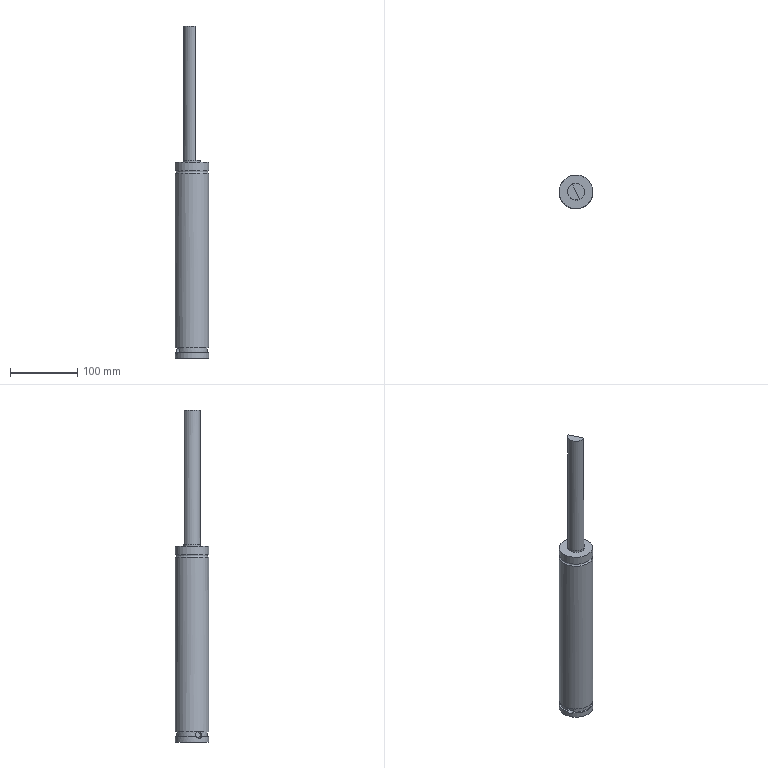Part | NX | features MAIN_BODY 2 | 1 solid | 16 faces | box 50.2 x 50.2 x 495 mm | volume 624869 mm3 | plane 8 | cylinder 7 | torus 1 | commonest cylinder face diameters 50.2 x3 9.72 x1 24.98 x1 25 x1 46.2 x1
STEP:
#1=CARTESIAN_POINT('',(178.732,295.899,-605.));
#2=VERTEX_POINT('',#1);
#3=CARTESIAN_POINT('',(177.181,299.227,-605.));
#4=VERTEX_POINT('',#3);
#5=CARTESIAN_POINT('',(200.644,308.142,-605.));
#6=DIRECTION('',(0.,0.,-1.));
#7=DIRECTION('',(0.9063,0.4226,0.));
#8=AXIS2_PLACEMENT_3D('',#5,#6,#7);
#9=CIRCLE('',#8,25.1);
#10=EDGE_CURVE('',#2,#4,#9,.F.);
#11=ORIENTED_EDGE('',*,*,#10,.T.);
#12=CARTESIAN_POINT('',(177.181,299.227,-605.));
#13=CARTESIAN_POINT('',(177.597,298.13,-604.523));
#14=CARTESIAN_POINT('',(178.16,296.923,-604.523));
#15=CARTESIAN_POINT('',(178.732,295.899,-605.));
#16=B_SPLINE_CURVE_WITH_KNOTS('',3,(#12,#13,#14,#15),.UNSPECIFIED.,.F.,.F.,(4,4),(0.,0.003746),.UNSPECIFIED.);
#17=EDGE_CURVE('',#4,#2,#16,.T.);
#18=ORIENTED_EDGE('',*,*,#17,.T.);
#19=EDGE_LOOP('',(#11,#18));
#20=FACE_BOUND('',#19,.T.);
#21=CARTESIAN_POINT('',(223.392,318.75,-344.5));
#22=VERTEX_POINT('',#21);
#23=CARTESIAN_POINT('',(200.644,308.142,-344.5));
#24=DIRECTION('',(0.,0.,-1.));
#25=DIRECTION('',(0.9063,0.4226,0.));
#26=AXIS2_PLACEMENT_3D('',#23,#24,#25);
#27=CIRCLE('',#26,25.1);
#28=EDGE_CURVE('',#22,#22,#27,.T.);
#29=ORIENTED_EDGE('',*,*,#28,.T.);
#30=EDGE_LOOP('',(#29));
#31=FACE_BOUND('',#30,.T.);
#32=CARTESIAN_POINT('',(200.644,308.142,-328.));
#33=DIRECTION('',(0.,0.,-1.));
#34=DIRECTION('',(0.9063,0.4226,0.));
#35=AXIS2_PLACEMENT_3D('',#32,#33,#34);
#36=CYLINDRICAL_SURFACE('',#35,25.1);
#37=ADVANCED_FACE('',(#20,#31),#36,.T.);
#38=CARTESIAN_POINT('',(177.896,297.535,-328.));
#39=VERTEX_POINT('',#38);
#40=CARTESIAN_POINT('',(200.644,308.142,-328.));
#41=DIRECTION('',(0.,0.,1.));
#42=DIRECTION('',(-0.9063,-0.4226,0.));
#43=AXIS2_PLACEMENT_3D('',#40,#41,#42);
#44=CIRCLE('',#43,25.1);
#45=EDGE_CURVE('',#39,#39,#44,.T.);
#46=ORIENTED_EDGE('',*,*,#45,.T.);
#47=EDGE_LOOP('',(#46));
#48=FACE_BOUND('',#47,.T.);
#49=CARTESIAN_POINT('',(189.315,302.86,-328.));
#50=VERTEX_POINT('',#49);
#51=CARTESIAN_POINT('',(200.644,308.142,-328.));
#52=DIRECTION('',(0.,0.,1.));
#53=DIRECTION('',(-0.9063,-0.4226,0.));
#54=AXIS2_PLACEMENT_3D('',#51,#52,#53);
#55=CIRCLE('',#54,12.5);
#56=EDGE_CURVE('',#50,#50,#55,.T.);
#57=ORIENTED_EDGE('',*,*,#56,.F.);
#58=EDGE_LOOP('',(#57));
#59=FACE_BOUND('',#58,.T.);
#60=CARTESIAN_POINT('',(200.644,308.142,-328.));
#61=DIRECTION('',(0.,0.,1.));
#62=DIRECTION('',(-0.9063,-0.4226,0.));
#63=AXIS2_PLACEMENT_3D('',#60,#61,#62);
#64=PLANE('',#63);
#65=ADVANCED_FACE('',(#48,#59),#64,.T.);
#66=CARTESIAN_POINT('',(223.392,318.75,-340.5));
#67=VERTEX_POINT('',#66);
#68=CARTESIAN_POINT('',(200.644,308.142,-340.5));
#69=DIRECTION('',(0.,0.,-1.));
#70=DIRECTION('',(0.9063,0.4226,0.));
#71=AXIS2_PLACEMENT_3D('',#68,#69,#70);
#72=CIRCLE('',#71,25.1);
#73=EDGE_CURVE('',#67,#67,#72,.F.);
#74=ORIENTED_EDGE('',*,*,#73,.T.);
#75=EDGE_LOOP('',(#74));
#76=FACE_BOUND('',#75,.T.);
#77=ORIENTED_EDGE('',*,*,#45,.F.);
#78=EDGE_LOOP('',(#77));
#79=FACE_BOUND('',#78,.T.);
#80=CARTESIAN_POINT('',(200.644,308.142,-328.));
#81=DIRECTION('',(0.,0.,-1.));
#82=DIRECTION('',(0.9063,0.4226,0.));
#83=AXIS2_PLACEMENT_3D('',#80,#81,#82);
#84=CYLINDRICAL_SURFACE('',#83,25.1);
#85=ADVANCED_FACE('',(#76,#79),#84,.T.);
#86=CARTESIAN_POINT('',(195.363,319.467,-325.));
#87=VERTEX_POINT('',#86);
#88=CARTESIAN_POINT('',(205.925,296.818,-325.));
#89=VERTEX_POINT('',#88);
#90=CARTESIAN_POINT('',(205.927,296.813,-325.));
#91=CARTESIAN_POINT('',(202.961,295.43,-325.));
#92=CARTESIAN_POINT('',(195.91,295.127,-325.));
#93=CARTESIAN_POINT('',(188.088,302.287,-325.));
#94=CARTESIAN_POINT('',(187.63,312.882,-325.));
#95=CARTESIAN_POINT('',(192.395,318.088,-325.));
#96=CARTESIAN_POINT('',(195.361,319.471,-325.));
#97=B_SPLINE_CURVE_WITH_KNOTS('',3,(#90,#91,#92,#93,#94,#95,#96),.UNSPECIFIED.,.F.,.F.,(4,1,1,1,4),(0.75,0.875,1.,1.125,1.25),.UNSPECIFIED.);
#98=EDGE_CURVE('',#87,#89,#97,.F.);
#99=ORIENTED_EDGE('',*,*,#98,.F.);
#100=CARTESIAN_POINT('',(195.365,319.462,-325.));
#101=CARTESIAN_POINT('',(196.867,320.162,-325.));
#102=CARTESIAN_POINT('',(200.075,320.939,-325.));
#103=CARTESIAN_POINT('',(206.686,319.944,-325.));
#104=CARTESIAN_POINT('',(213.188,313.992,-325.));
#105=CARTESIAN_POINT('',(213.569,305.185,-325.));
#106=CARTESIAN_POINT('',(210.081,299.481,-325.));
#107=CARTESIAN_POINT('',(207.424,297.523,-325.));
#108=CARTESIAN_POINT('',(205.922,296.822,-325.));
#109=B_SPLINE_CURVE_WITH_KNOTS('',3,(#100,#101,#102,#103,#104,#105,#106,#107,#108),.UNSPECIFIED.,.F.,.F.,(4,1,1,1,1,1,4),(0.,0.125,0.25,0.5,0.75,0.875,1.),.UNSPECIFIED.);
#110=EDGE_CURVE('',#87,#89,#109,.T.);
#111=ORIENTED_EDGE('',*,*,#110,.T.);
#112=EDGE_LOOP('',(#99,#111));
#113=FACE_BOUND('',#112,.T.);
#114=ORIENTED_EDGE('',*,*,#56,.T.);
#115=EDGE_LOOP('',(#114));
#116=FACE_BOUND('',#115,.T.);
#117=CARTESIAN_POINT('',(200.644,308.142,-325.));
#118=DIRECTION('',(0.,0.,-1.));
#119=DIRECTION('',(0.9063,0.4226,0.));
#120=AXIS2_PLACEMENT_3D('',#117,#118,#119);
#121=CYLINDRICAL_SURFACE('',#120,12.5);
#122=ADVANCED_FACE('',(#113,#116),#121,.T.);
#123=ORIENTED_EDGE('',*,*,#73,.F.);
#124=EDGE_LOOP('',(#123));
#125=FACE_BOUND('',#124,.T.);
#126=ORIENTED_EDGE('',*,*,#28,.F.);
#127=EDGE_LOOP('',(#126));
#128=FACE_BOUND('',#127,.T.);
#129=CARTESIAN_POINT('',(200.644,308.142,-342.5));
#130=DIRECTION('',(0.,0.,-1.));
#131=DIRECTION('',(0.9063,0.4226,0.));
#132=AXIS2_PLACEMENT_3D('',#129,#130,#131);
#133=TOROIDAL_SURFACE('',#132,25.1,2.);
#134=ADVANCED_FACE('',(#125,#128),#133,.F.);
#135=ORIENTED_EDGE('',*,*,#10,.F.);
#136=CARTESIAN_POINT('',(180.55,296.747,-605.));
#137=VERTEX_POINT('',#136);
#138=CARTESIAN_POINT('',(185.469,299.04,-605.));
#139=DIRECTION('',(-0.9063,-0.4226,0.));
#140=VECTOR('',#139,1000.);
#141=LINE('',#138,#140);
#142=EDGE_CURVE('',#2,#137,#141,.F.);
#143=ORIENTED_EDGE('',*,*,#142,.T.);
#144=CARTESIAN_POINT('',(178.999,300.074,-605.));
#145=VERTEX_POINT('',#144);
#146=CARTESIAN_POINT('',(200.644,308.142,-605.));
#147=DIRECTION('',(0.,0.,1.));
#148=DIRECTION('',(-0.9063,-0.4226,0.));
#149=AXIS2_PLACEMENT_3D('',#146,#147,#148);
#150=CIRCLE('',#149,23.1);
#151=EDGE_CURVE('',#137,#145,#150,.T.);
#152=ORIENTED_EDGE('',*,*,#151,.T.);
#153=CARTESIAN_POINT('',(183.917,302.368,-605.));
#154=DIRECTION('',(-0.9063,-0.4226,0.));
#155=VECTOR('',#154,1000.);
#156=LINE('',#153,#155);
#157=EDGE_CURVE('',#145,#4,#156,.T.);
#158=ORIENTED_EDGE('',*,*,#157,.T.);
#159=EDGE_LOOP('',(#135,#143,#152,#158));
#160=FACE_BOUND('',#159,.T.);
#161=CARTESIAN_POINT('',(200.644,308.142,-605.));
#162=DIRECTION('',(0.,0.,-1.));
#163=DIRECTION('',(0.9063,0.4226,0.));
#164=AXIS2_PLACEMENT_3D('',#161,#162,#163);
#165=PLANE('',#164);
#166=ADVANCED_FACE('',(#160),#165,.T.);
#167=CARTESIAN_POINT('',(181.813,294.763,-612.));
#168=VERTEX_POINT('',#167);
#169=CARTESIAN_POINT('',(178.29,302.317,-612.));
#170=VERTEX_POINT('',#169);
#171=CARTESIAN_POINT('',(200.644,308.142,-612.));
#172=DIRECTION('',(0.,0.,1.));
#173=DIRECTION('',(-0.9063,-0.4226,0.));
#174=AXIS2_PLACEMENT_3D('',#171,#172,#173);
#175=CIRCLE('',#174,23.1);
#176=EDGE_CURVE('',#168,#170,#175,.T.);
#177=ORIENTED_EDGE('',*,*,#176,.F.);
#178=CARTESIAN_POINT('',(179.973,293.905,-612.));
#179=VERTEX_POINT('',#178);
#180=CARTESIAN_POINT('',(186.454,296.927,-612.));
#181=DIRECTION('',(-0.9063,-0.4226,0.));
#182=VECTOR('',#181,1000.);
#183=LINE('',#180,#182);
#184=EDGE_CURVE('',#168,#179,#183,.T.);
#185=ORIENTED_EDGE('',*,*,#184,.T.);
#186=CARTESIAN_POINT('',(176.45,301.459,-612.));
#187=VERTEX_POINT('',#186);
#188=CARTESIAN_POINT('',(200.644,308.142,-612.));
#189=DIRECTION('',(0.,0.,-1.));
#190=DIRECTION('',(0.9063,0.4226,0.));
#191=AXIS2_PLACEMENT_3D('',#188,#189,#190);
#192=CIRCLE('',#191,25.1);
#193=EDGE_CURVE('',#187,#179,#192,.T.);
#194=ORIENTED_EDGE('',*,*,#193,.F.);
#195=CARTESIAN_POINT('',(182.932,304.481,-612.));
#196=DIRECTION('',(-0.9063,-0.4226,0.));
#197=VECTOR('',#196,1000.);
#198=LINE('',#195,#197);
#199=EDGE_CURVE('',#187,#170,#198,.F.);
#200=ORIENTED_EDGE('',*,*,#199,.T.);
#201=EDGE_LOOP('',(#177,#185,#194,#200));
#202=FACE_BOUND('',#201,.T.);
#203=CARTESIAN_POINT('',(200.644,308.142,-612.));
#204=DIRECTION('',(0.,0.,-1.));
#205=DIRECTION('',(0.9063,0.4226,0.));
#206=AXIS2_PLACEMENT_3D('',#203,#204,#205);
#207=PLANE('',#206);
#208=ADVANCED_FACE('',(#202),#207,.F.);
#209=CARTESIAN_POINT('',(181.813,294.763,-612.));
#210=CARTESIAN_POINT('',(182.239,294.163,-610.794));
#211=CARTESIAN_POINT('',(182.437,293.911,-607.757));
#212=CARTESIAN_POINT('',(181.196,295.608,-605.532));
#213=CARTESIAN_POINT('',(180.55,296.747,-605.));
#214=B_SPLINE_CURVE_WITH_KNOTS('',3,(#209,#210,#211,#212,#213),.UNSPECIFIED.,.F.,.F.,(4,1,4),(0.,0.00418,0.00836),.UNSPECIFIED.);
#215=EDGE_CURVE('',#168,#137,#214,.T.);
#216=ORIENTED_EDGE('',*,*,#215,.F.);
#217=ORIENTED_EDGE('',*,*,#176,.T.);
#218=CARTESIAN_POINT('',(178.999,300.074,-605.));
#219=CARTESIAN_POINT('',(178.541,301.301,-605.532));
#220=CARTESIAN_POINT('',(178.04,303.34,-607.75));
#221=CARTESIAN_POINT('',(178.105,303.029,-610.793));
#222=CARTESIAN_POINT('',(178.29,302.317,-612.));
#223=B_SPLINE_CURVE_WITH_KNOTS('',3,(#218,#219,#220,#221,#222),.UNSPECIFIED.,.F.,.F.,(4,1,4),(0.,0.00418,0.008359),.UNSPECIFIED.);
#224=EDGE_CURVE('',#145,#170,#223,.T.);
#225=ORIENTED_EDGE('',*,*,#224,.F.);
#226=ORIENTED_EDGE('',*,*,#151,.F.);
#227=EDGE_LOOP('',(#216,#217,#225,#226));
#228=FACE_BOUND('',#227,.T.);
#229=CARTESIAN_POINT('',(200.644,308.142,-612.));
#230=DIRECTION('',(0.,0.,1.));
#231=DIRECTION('',(-0.9063,-0.4226,0.));
#232=AXIS2_PLACEMENT_3D('',#229,#230,#231);
#233=CYLINDRICAL_SURFACE('',#232,23.1);
#234=ADVANCED_FACE('',(#228),#233,.T.);
#235=CARTESIAN_POINT('',(177.896,297.535,-620.));
#236=VERTEX_POINT('',#235);
#237=CARTESIAN_POINT('',(200.644,308.142,-620.));
#238=DIRECTION('',(0.,0.,1.));
#239=DIRECTION('',(-0.9063,-0.4226,0.));
#240=AXIS2_PLACEMENT_3D('',#237,#238,#239);
#241=CIRCLE('',#240,25.1);
#242=EDGE_CURVE('',#236,#236,#241,.T.);
#243=ORIENTED_EDGE('',*,*,#242,.F.);
#244=EDGE_LOOP('',(#243));
#245=FACE_BOUND('',#244,.T.);
#246=CARTESIAN_POINT('',(200.644,308.142,-620.));
#247=DIRECTION('',(0.,0.,1.));
#248=DIRECTION('',(-0.9063,-0.4226,0.));
#249=AXIS2_PLACEMENT_3D('',#246,#247,#248);
#250=PLANE('',#249);
#251=ADVANCED_FACE('',(#245),#250,.F.);
#252=ORIENTED_EDGE('',*,*,#193,.T.);
#253=CARTESIAN_POINT('',(179.973,293.905,-612.));
#254=CARTESIAN_POINT('',(179.474,294.628,-613.445));
#255=CARTESIAN_POINT('',(177.712,297.449,-615.275));
#256=CARTESIAN_POINT('',(176.684,300.612,-613.445));
#257=CARTESIAN_POINT('',(176.45,301.459,-612.));
#258=B_SPLINE_CURVE_WITH_KNOTS('',3,(#253,#254,#255,#256,#257),.UNSPECIFIED.,.F.,.F.,(4,1,4),(-0.005001,0.000000028,0.005001),.UNSPECIFIED.);
#259=EDGE_CURVE('',#179,#187,#258,.T.);
#260=ORIENTED_EDGE('',*,*,#259,.T.);
#261=EDGE_LOOP('',(#252,#260));
#262=FACE_BOUND('',#261,.T.);
#263=ORIENTED_EDGE('',*,*,#242,.T.);
#264=EDGE_LOOP('',(#263));
#265=FACE_BOUND('',#264,.T.);
#266=CARTESIAN_POINT('',(200.644,308.142,-328.));
#267=DIRECTION('',(0.,0.,-1.));
#268=DIRECTION('',(0.9063,0.4226,0.));
#269=AXIS2_PLACEMENT_3D('',#266,#267,#268);
#270=CYLINDRICAL_SURFACE('',#269,25.1);
#271=ADVANCED_FACE('',(#262,#265),#270,.T.);
#272=CARTESIAN_POINT('',(186.747,296.299,-609.5));
#273=VERTEX_POINT('',#272);
#274=CARTESIAN_POINT('',(184.693,300.704,-609.5));
#275=DIRECTION('',(-0.9063,-0.4226,0.));
#276=DIRECTION('',(0.4226,-0.9063,0.));
#277=AXIS2_PLACEMENT_3D('',#274,#275,#276);
#278=CIRCLE('',#277,4.86);
#279=EDGE_CURVE('',#273,#273,#278,.T.);
#280=ORIENTED_EDGE('',*,*,#279,.F.);
#281=EDGE_LOOP('',(#280));
#282=FACE_BOUND('',#281,.T.);
#283=ORIENTED_EDGE('',*,*,#157,.F.);
#284=ORIENTED_EDGE('',*,*,#224,.T.);
#285=ORIENTED_EDGE('',*,*,#199,.F.);
#286=ORIENTED_EDGE('',*,*,#259,.F.);
#287=ORIENTED_EDGE('',*,*,#184,.F.);
#288=ORIENTED_EDGE('',*,*,#215,.T.);
#289=ORIENTED_EDGE('',*,*,#142,.F.);
#290=ORIENTED_EDGE('',*,*,#17,.F.);
#291=EDGE_LOOP('',(#283,#284,#285,#286,#287,#288,#289,#290));
#292=FACE_BOUND('',#291,.T.);
#293=CARTESIAN_POINT('',(184.693,300.704,-609.5));
#294=DIRECTION('',(-0.9063,-0.4226,0.));
#295=DIRECTION('',(0.,0.,-1.));
#296=AXIS2_PLACEMENT_3D('',#293,#294,#295);
#297=CYLINDRICAL_SURFACE('',#296,4.86);
#298=ADVANCED_FACE('',(#282,#292),#297,.F.);
#299=ORIENTED_EDGE('',*,*,#279,.T.);
#300=EDGE_LOOP('',(#299));
#301=FACE_BOUND('',#300,.T.);
#302=CARTESIAN_POINT('',(184.693,300.704,-609.5));
#303=DIRECTION('',(-0.9063,-0.4226,0.));
#304=DIRECTION('',(0.,0.,-1.));
#305=AXIS2_PLACEMENT_3D('',#302,#303,#304);
#306=PLANE('',#305);
#307=ADVANCED_FACE('',(#301),#306,.T.);
#308=ORIENTED_EDGE('',*,*,#98,.T.);
#309=CARTESIAN_POINT('',(205.927,296.813,-125.));
#310=VERTEX_POINT('',#309);
#311=CARTESIAN_POINT('',(205.922,296.822,-125.));
#312=DIRECTION('',(0.,0.,-1.));
#313=VECTOR('',#312,1000.);
#314=LINE('',#311,#313);
#315=EDGE_CURVE('',#310,#89,#314,.T.);
#316=ORIENTED_EDGE('',*,*,#315,.F.);
#317=CARTESIAN_POINT('',(195.361,319.471,-125.));
#318=VERTEX_POINT('',#317);
#319=CARTESIAN_POINT('',(200.644,308.142,-125.));
#320=DIRECTION('',(0.,0.,1.));
#321=DIRECTION('',(-0.9063,-0.4226,0.));
#322=AXIS2_PLACEMENT_3D('',#319,#320,#321);
#323=CIRCLE('',#322,12.49);
#324=EDGE_CURVE('',#318,#310,#323,.T.);
#325=ORIENTED_EDGE('',*,*,#324,.F.);
#326=CARTESIAN_POINT('',(195.365,319.462,-315.));
#327=DIRECTION('',(0.,0.,-1.));
#328=VECTOR('',#327,1000.);
#329=LINE('',#326,#328);
#330=EDGE_CURVE('',#87,#318,#329,.F.);
#331=ORIENTED_EDGE('',*,*,#330,.F.);
#332=EDGE_LOOP('',(#308,#316,#325,#331));
#333=FACE_BOUND('',#332,.T.);
#334=CARTESIAN_POINT('',(200.644,308.142,-125.));
#335=DIRECTION('',(0.,0.,-1.));
#336=DIRECTION('',(0.9063,0.4226,0.));
#337=AXIS2_PLACEMENT_3D('',#334,#335,#336);
#338=CYLINDRICAL_SURFACE('',#337,12.49);
#339=ADVANCED_FACE('',(#333),#338,.T.);
#340=ORIENTED_EDGE('',*,*,#324,.T.);
#341=CARTESIAN_POINT('',(277.646,143.011,-125.));
#342=DIRECTION('',(-0.4226,0.9063,0.));
#343=VECTOR('',#342,1000.);
#344=LINE('',#341,#343);
#345=EDGE_CURVE('',#310,#318,#344,.T.);
#346=ORIENTED_EDGE('',*,*,#345,.T.);
#347=EDGE_LOOP('',(#340,#346));
#348=FACE_BOUND('',#347,.T.);
#349=CARTESIAN_POINT('',(200.644,308.142,-125.));
#350=DIRECTION('',(0.,0.,1.));
#351=DIRECTION('',(-0.9063,-0.4226,0.));
#352=AXIS2_PLACEMENT_3D('',#349,#350,#351);
#353=PLANE('',#352);
#354=ADVANCED_FACE('',(#348),#353,.T.);
#355=CARTESIAN_POINT('',(277.646,143.011,-325.));
#356=DIRECTION('',(-0.4226,0.9063,0.));
#357=VECTOR('',#356,1000.);
#358=LINE('',#355,#357);
#359=EDGE_CURVE('',#89,#87,#358,.T.);
#360=ORIENTED_EDGE('',*,*,#359,.F.);
#361=ORIENTED_EDGE('',*,*,#110,.F.);
#362=EDGE_LOOP('',(#360,#361));
#363=FACE_BOUND('',#362,.T.);
#364=CARTESIAN_POINT('',(277.646,143.011,-325.));
#365=DIRECTION('',(0.,0.,-1.));
#366=DIRECTION('',(0.9063,0.4226,0.));
#367=AXIS2_PLACEMENT_3D('',#364,#365,#366);
#368=PLANE('',#367);
#369=ADVANCED_FACE('',(#363),#368,.F.);
#370=ORIENTED_EDGE('',*,*,#315,.T.);
#371=ORIENTED_EDGE('',*,*,#359,.T.);
#372=ORIENTED_EDGE('',*,*,#330,.T.);
#373=ORIENTED_EDGE('',*,*,#345,.F.);
#374=EDGE_LOOP('',(#370,#371,#372,#373));
#375=FACE_BOUND('',#374,.T.);
#376=CARTESIAN_POINT('',(277.646,143.011,-315.));
#377=DIRECTION('',(0.9063,0.4226,0.));
#378=DIRECTION('',(-0.4226,0.9063,0.));
#379=AXIS2_PLACEMENT_3D('',#376,#377,#378);
#380=PLANE('',#379);
#381=ADVANCED_FACE('',(#375),#380,.T.);
#382=CLOSED_SHELL('',(#37,#65,#85,#122,#134,#166,#208,#234,#251,#271,#298,#307,#339,#354,#369,#381));
#383=MANIFOLD_SOLID_BREP('',#382);
#384=(LENGTH_UNIT()NAMED_UNIT(*)SI_UNIT(.MILLI.,.METRE.));
#385=UNCERTAINTY_MEASURE_WITH_UNIT(LENGTH_MEASURE(0.0508),#384,'','');
#386=(NAMED_UNIT(*)PLANE_ANGLE_UNIT()SI_UNIT($,.RADIAN.));
#387=(NAMED_UNIT(*)SI_UNIT($,.STERADIAN.)SOLID_ANGLE_UNIT());
#388=(GEOMETRIC_REPRESENTATION_CONTEXT(3)GLOBAL_UNCERTAINTY_ASSIGNED_CONTEXT((#385))GLOBAL_UNIT_ASSIGNED_CONTEXT((#384,#386,#387))REPRESENTATION_CONTEXT('',''));
#389=ADVANCED_BREP_SHAPE_REPRESENTATION('',(#383),#388);